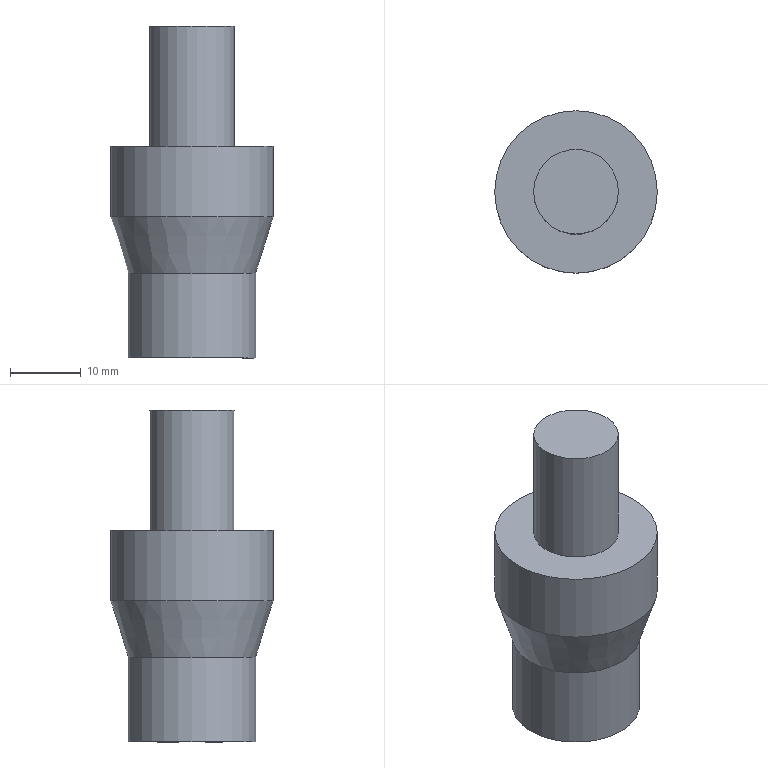Part | NX | features solid 2 | 1 solid | 7 faces | box 23 x 23 x 47 mm | volume 11785 mm3 | plane 3 | cylinder 3 | cone 1 | commonest cylinder face diameters 12 x1 18 x1 23 x1
STEP:
#1=CARTESIAN_POINT('',(-36.,-335.,112.));
#2=VERTEX_POINT('',#1);
#3=CARTESIAN_POINT('',(-30.,-335.,112.));
#4=DIRECTION('',(0.,0.,1.));
#5=DIRECTION('',(-1.,0.,0.));
#6=AXIS2_PLACEMENT_3D('',#3,#4,#5);
#7=CIRCLE('',#6,6.);
#8=EDGE_CURVE('',#2,#2,#7,.T.);
#9=ORIENTED_EDGE('',*,*,#8,.T.);
#10=EDGE_LOOP('',(#9));
#11=FACE_BOUND('',#10,.T.);
#12=CARTESIAN_POINT('',(-30.,-335.,112.));
#13=DIRECTION('',(0.,0.,1.));
#14=DIRECTION('',(1.,0.,0.));
#15=AXIS2_PLACEMENT_3D('',#12,#13,#14);
#16=PLANE('',#15);
#17=ADVANCED_FACE('',(#11),#16,.T.);
#18=CARTESIAN_POINT('',(-18.5,-335.,95.));
#19=VERTEX_POINT('',#18);
#20=CARTESIAN_POINT('',(-30.,-335.,95.));
#21=DIRECTION('',(0.,0.,1.));
#22=DIRECTION('',(1.,0.,0.));
#23=AXIS2_PLACEMENT_3D('',#20,#21,#22);
#24=CIRCLE('',#23,11.5);
#25=EDGE_CURVE('',#19,#19,#24,.T.);
#26=ORIENTED_EDGE('',*,*,#25,.T.);
#27=EDGE_LOOP('',(#26));
#28=FACE_BOUND('',#27,.T.);
#29=CARTESIAN_POINT('',(-24.,-335.,95.));
#30=VERTEX_POINT('',#29);
#31=CARTESIAN_POINT('',(-30.,-335.,95.));
#32=DIRECTION('',(0.,0.,1.));
#33=DIRECTION('',(1.,0.,0.));
#34=AXIS2_PLACEMENT_3D('',#31,#32,#33);
#35=CIRCLE('',#34,6.);
#36=EDGE_CURVE('',#30,#30,#35,.T.);
#37=ORIENTED_EDGE('',*,*,#36,.F.);
#38=EDGE_LOOP('',(#37));
#39=FACE_BOUND('',#38,.T.);
#40=CARTESIAN_POINT('',(-24.,-335.,95.));
#41=DIRECTION('',(0.,0.,1.));
#42=DIRECTION('',(1.,0.,0.));
#43=AXIS2_PLACEMENT_3D('',#40,#41,#42);
#44=PLANE('',#43);
#45=ADVANCED_FACE('',(#28,#39),#44,.T.);
#46=CARTESIAN_POINT('',(-21.,-335.,77.));
#47=VERTEX_POINT('',#46);
#48=CARTESIAN_POINT('',(-30.,-335.,77.));
#49=DIRECTION('',(0.,0.,1.));
#50=DIRECTION('',(1.,0.,0.));
#51=AXIS2_PLACEMENT_3D('',#48,#49,#50);
#52=CIRCLE('',#51,9.);
#53=EDGE_CURVE('',#47,#47,#52,.T.);
#54=ORIENTED_EDGE('',*,*,#53,.T.);
#55=EDGE_LOOP('',(#54));
#56=FACE_BOUND('',#55,.T.);
#57=CARTESIAN_POINT('',(-18.5,-335.,85.));
#58=VERTEX_POINT('',#57);
#59=CARTESIAN_POINT('',(-30.,-335.,85.));
#60=DIRECTION('',(0.,0.,1.));
#61=DIRECTION('',(1.,0.,0.));
#62=AXIS2_PLACEMENT_3D('',#59,#60,#61);
#63=CIRCLE('',#62,11.5);
#64=EDGE_CURVE('',#58,#58,#63,.T.);
#65=ORIENTED_EDGE('',*,*,#64,.F.);
#66=EDGE_LOOP('',(#65));
#67=FACE_BOUND('',#66,.T.);
#68=CARTESIAN_POINT('',(-30.,-335.,85.));
#69=DIRECTION('',(0.,0.,1.));
#70=DIRECTION('',(1.,0.,0.));
#71=AXIS2_PLACEMENT_3D('',#68,#69,#70);
#72=CONICAL_SURFACE('',#71,11.5,0.3029);
#73=ADVANCED_FACE('',(#56,#67),#72,.T.);
#74=ORIENTED_EDGE('',*,*,#8,.F.);
#75=EDGE_LOOP('',(#74));
#76=FACE_BOUND('',#75,.T.);
#77=ORIENTED_EDGE('',*,*,#36,.T.);
#78=EDGE_LOOP('',(#77));
#79=FACE_BOUND('',#78,.T.);
#80=CARTESIAN_POINT('',(-30.,-335.,117.));
#81=DIRECTION('',(0.,0.,1.));
#82=DIRECTION('',(1.,0.,0.));
#83=AXIS2_PLACEMENT_3D('',#80,#81,#82);
#84=CYLINDRICAL_SURFACE('',#83,6.);
#85=ADVANCED_FACE('',(#76,#79),#84,.T.);
#86=ORIENTED_EDGE('',*,*,#25,.F.);
#87=EDGE_LOOP('',(#86));
#88=FACE_BOUND('',#87,.T.);
#89=ORIENTED_EDGE('',*,*,#64,.T.);
#90=EDGE_LOOP('',(#89));
#91=FACE_BOUND('',#90,.T.);
#92=CARTESIAN_POINT('',(-30.,-335.,117.));
#93=DIRECTION('',(0.,0.,1.));
#94=DIRECTION('',(1.,0.,0.));
#95=AXIS2_PLACEMENT_3D('',#92,#93,#94);
#96=CYLINDRICAL_SURFACE('',#95,11.5);
#97=ADVANCED_FACE('',(#88,#91),#96,.T.);
#98=ORIENTED_EDGE('',*,*,#53,.F.);
#99=EDGE_LOOP('',(#98));
#100=FACE_BOUND('',#99,.T.);
#101=CARTESIAN_POINT('',(-21.,-335.,65.));
#102=VERTEX_POINT('',#101);
#103=CARTESIAN_POINT('',(-30.,-335.,65.));
#104=DIRECTION('',(0.,0.,1.));
#105=DIRECTION('',(1.,0.,0.));
#106=AXIS2_PLACEMENT_3D('',#103,#104,#105);
#107=CIRCLE('',#106,9.);
#108=EDGE_CURVE('',#102,#102,#107,.T.);
#109=ORIENTED_EDGE('',*,*,#108,.T.);
#110=EDGE_LOOP('',(#109));
#111=FACE_BOUND('',#110,.T.);
#112=CARTESIAN_POINT('',(-30.,-335.,117.));
#113=DIRECTION('',(0.,0.,1.));
#114=DIRECTION('',(1.,0.,0.));
#115=AXIS2_PLACEMENT_3D('',#112,#113,#114);
#116=CYLINDRICAL_SURFACE('',#115,9.);
#117=ADVANCED_FACE('',(#100,#111),#116,.T.);
#118=ORIENTED_EDGE('',*,*,#108,.F.);
#119=EDGE_LOOP('',(#118));
#120=FACE_BOUND('',#119,.T.);
#121=CARTESIAN_POINT('',(-30.,-335.,65.));
#122=DIRECTION('',(0.,0.,1.));
#123=DIRECTION('',(1.,0.,0.));
#124=AXIS2_PLACEMENT_3D('',#121,#122,#123);
#125=PLANE('',#124);
#126=ADVANCED_FACE('',(#120),#125,.F.);
#127=CLOSED_SHELL('',(#17,#45,#73,#85,#97,#117,#126));
#128=MANIFOLD_SOLID_BREP('',#127);
#129=(LENGTH_UNIT()NAMED_UNIT(*)SI_UNIT(.MILLI.,.METRE.));
#130=UNCERTAINTY_MEASURE_WITH_UNIT(LENGTH_MEASURE(0.00001),#129,'','');
#131=(NAMED_UNIT(*)PLANE_ANGLE_UNIT()SI_UNIT($,.RADIAN.));
#132=(NAMED_UNIT(*)SI_UNIT($,.STERADIAN.)SOLID_ANGLE_UNIT());
#133=(GEOMETRIC_REPRESENTATION_CONTEXT(3)GLOBAL_UNCERTAINTY_ASSIGNED_CONTEXT((#130))GLOBAL_UNIT_ASSIGNED_CONTEXT((#129,#131,#132))REPRESENTATION_CONTEXT('',''));
#134=ADVANCED_BREP_SHAPE_REPRESENTATION('',(#128),#133);